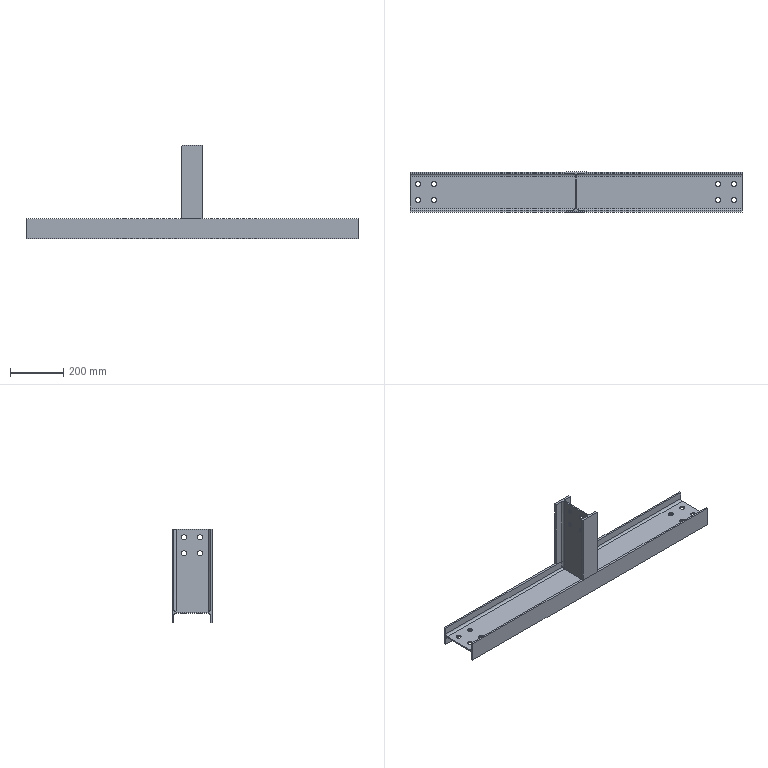Part | STEP file | Powder bin secondary beam 6 body_Default<As Machined> | 2 solids | 66 faces | box 1245 x 150 x 350 mm | volume 2721156 mm3 | plane 34 | cylinder 32 | commonest cylinder face diameters 19 x24 16 x8